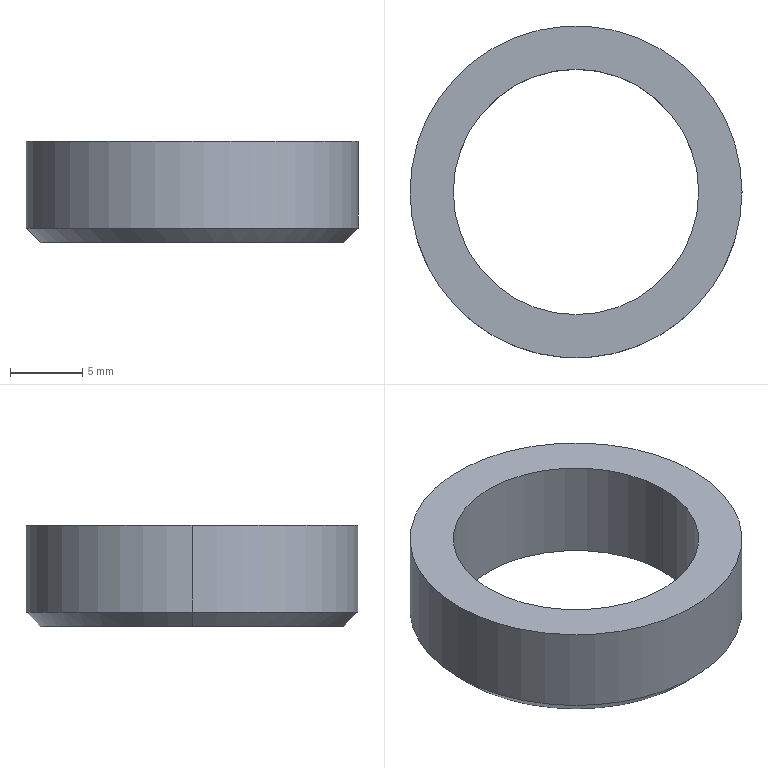Part | NX | features BREP 1 | 1 solid | 8 faces | box 23 x 23 x 7 mm | volume 1284 mm3 | cylinder 4 | cone 2 | plane 2 | commonest cylinder face diameters 17 x2 23 x2
STEP:
#1=CARTESIAN_POINT('',(-11.5,0.,-6.));
#2=VERTEX_POINT('',#1);
#3=CARTESIAN_POINT('',(-11.5,0.,0.));
#4=VERTEX_POINT('',#3);
#5=CARTESIAN_POINT('',(-11.5,0.,0.));
#6=DIRECTION('',(0.,0.,-1.));
#7=VECTOR('',#6,1000.);
#8=LINE('',#5,#7);
#9=EDGE_CURVE('',#2,#4,#8,.F.);
#10=ORIENTED_EDGE('',*,*,#9,.T.);
#11=CARTESIAN_POINT('',(11.5,0.,0.));
#12=VERTEX_POINT('',#11);
#13=CARTESIAN_POINT('',(0.,0.,0.));
#14=DIRECTION('',(0.,0.,1.));
#15=DIRECTION('',(1.,0.,0.));
#16=AXIS2_PLACEMENT_3D('',#13,#14,#15);
#17=CIRCLE('',#16,11.5);
#18=EDGE_CURVE('',#12,#4,#17,.T.);
#19=ORIENTED_EDGE('',*,*,#18,.F.);
#20=CARTESIAN_POINT('',(11.5,0.,-6.));
#21=VERTEX_POINT('',#20);
#22=CARTESIAN_POINT('',(11.5,0.,0.));
#23=DIRECTION('',(0.,0.,-1.));
#24=VECTOR('',#23,1000.);
#25=LINE('',#22,#24);
#26=EDGE_CURVE('',#21,#12,#25,.F.);
#27=ORIENTED_EDGE('',*,*,#26,.F.);
#28=CARTESIAN_POINT('',(0.,0.,-6.));
#29=DIRECTION('',(0.,0.,-1.));
#30=DIRECTION('',(-1.,0.,0.));
#31=AXIS2_PLACEMENT_3D('',#28,#29,#30);
#32=CIRCLE('',#31,11.5);
#33=EDGE_CURVE('',#2,#21,#32,.T.);
#34=ORIENTED_EDGE('',*,*,#33,.F.);
#35=EDGE_LOOP('',(#10,#19,#27,#34));
#36=FACE_BOUND('',#35,.T.);
#37=CARTESIAN_POINT('',(0.,0.,-7.));
#38=DIRECTION('',(0.,0.,1.));
#39=DIRECTION('',(-1.,0.,0.));
#40=AXIS2_PLACEMENT_3D('',#37,#38,#39);
#41=CYLINDRICAL_SURFACE('',#40,11.5);
#42=ADVANCED_FACE('',(#36),#41,.T.);
#43=CARTESIAN_POINT('',(-10.5,0.,-7.));
#44=VERTEX_POINT('',#43);
#45=CARTESIAN_POINT('',(-11.5,0.,-6.));
#46=DIRECTION('',(0.7071,0.,-0.7071));
#47=VECTOR('',#46,1000.);
#48=LINE('',#45,#47);
#49=EDGE_CURVE('',#44,#2,#48,.F.);
#50=ORIENTED_EDGE('',*,*,#49,.T.);
#51=ORIENTED_EDGE('',*,*,#33,.T.);
#52=CARTESIAN_POINT('',(10.5,0.,-7.));
#53=VERTEX_POINT('',#52);
#54=CARTESIAN_POINT('',(11.5,0.,-6.));
#55=DIRECTION('',(-0.7071,0.,-0.7071));
#56=VECTOR('',#55,1000.);
#57=LINE('',#54,#56);
#58=EDGE_CURVE('',#53,#21,#57,.F.);
#59=ORIENTED_EDGE('',*,*,#58,.F.);
#60=CARTESIAN_POINT('',(0.,0.,-7.));
#61=DIRECTION('',(0.,0.,-1.));
#62=DIRECTION('',(-1.,0.,0.));
#63=AXIS2_PLACEMENT_3D('',#60,#61,#62);
#64=CIRCLE('',#63,10.5);
#65=EDGE_CURVE('',#44,#53,#64,.T.);
#66=ORIENTED_EDGE('',*,*,#65,.F.);
#67=EDGE_LOOP('',(#50,#51,#59,#66));
#68=FACE_BOUND('',#67,.T.);
#69=CARTESIAN_POINT('',(0.,0.,-6.5));
#70=DIRECTION('',(0.,0.,1.));
#71=DIRECTION('',(-1.,0.,0.));
#72=AXIS2_PLACEMENT_3D('',#69,#70,#71);
#73=CONICAL_SURFACE('',#72,11.,0.7854);
#74=ADVANCED_FACE('',(#68),#73,.T.);
#75=ORIENTED_EDGE('',*,*,#65,.T.);
#76=CARTESIAN_POINT('',(0.,0.,-7.));
#77=DIRECTION('',(0.,0.,-1.));
#78=DIRECTION('',(1.,0.,0.));
#79=AXIS2_PLACEMENT_3D('',#76,#77,#78);
#80=CIRCLE('',#79,10.5);
#81=EDGE_CURVE('',#53,#44,#80,.T.);
#82=ORIENTED_EDGE('',*,*,#81,.T.);
#83=EDGE_LOOP('',(#75,#82));
#84=FACE_BOUND('',#83,.T.);
#85=CARTESIAN_POINT('',(8.5,0.,-7.));
#86=VERTEX_POINT('',#85);
#87=CARTESIAN_POINT('',(-8.5,0.,-7.));
#88=VERTEX_POINT('',#87);
#89=CARTESIAN_POINT('',(0.,0.,-7.));
#90=DIRECTION('',(0.,0.,1.));
#91=DIRECTION('',(1.,0.,0.));
#92=AXIS2_PLACEMENT_3D('',#89,#90,#91);
#93=CIRCLE('',#92,8.5);
#94=EDGE_CURVE('',#86,#88,#93,.T.);
#95=ORIENTED_EDGE('',*,*,#94,.T.);
#96=CARTESIAN_POINT('',(0.,0.,-7.));
#97=DIRECTION('',(0.,0.,1.));
#98=DIRECTION('',(-1.,0.,0.));
#99=AXIS2_PLACEMENT_3D('',#96,#97,#98);
#100=CIRCLE('',#99,8.5);
#101=EDGE_CURVE('',#88,#86,#100,.T.);
#102=ORIENTED_EDGE('',*,*,#101,.T.);
#103=EDGE_LOOP('',(#95,#102));
#104=FACE_BOUND('',#103,.T.);
#105=CARTESIAN_POINT('',(0.,0.,-7.));
#106=DIRECTION('',(0.,0.,-1.));
#107=DIRECTION('',(1.,0.,0.));
#108=AXIS2_PLACEMENT_3D('',#105,#106,#107);
#109=PLANE('',#108);
#110=ADVANCED_FACE('',(#84,#104),#109,.T.);
#111=ORIENTED_EDGE('',*,*,#81,.F.);
#112=ORIENTED_EDGE('',*,*,#58,.T.);
#113=CARTESIAN_POINT('',(0.,0.,-6.));
#114=DIRECTION('',(0.,0.,-1.));
#115=DIRECTION('',(1.,0.,0.));
#116=AXIS2_PLACEMENT_3D('',#113,#114,#115);
#117=CIRCLE('',#116,11.5);
#118=EDGE_CURVE('',#21,#2,#117,.T.);
#119=ORIENTED_EDGE('',*,*,#118,.T.);
#120=ORIENTED_EDGE('',*,*,#49,.F.);
#121=EDGE_LOOP('',(#111,#112,#119,#120));
#122=FACE_BOUND('',#121,.T.);
#123=CARTESIAN_POINT('',(0.,0.,-6.5));
#124=DIRECTION('',(0.,0.,1.));
#125=DIRECTION('',(-1.,0.,0.));
#126=AXIS2_PLACEMENT_3D('',#123,#124,#125);
#127=CONICAL_SURFACE('',#126,11.,0.7854);
#128=ADVANCED_FACE('',(#122),#127,.T.);
#129=ORIENTED_EDGE('',*,*,#118,.F.);
#130=ORIENTED_EDGE('',*,*,#26,.T.);
#131=CARTESIAN_POINT('',(0.,0.,0.));
#132=DIRECTION('',(0.,0.,1.));
#133=DIRECTION('',(-1.,0.,0.));
#134=AXIS2_PLACEMENT_3D('',#131,#132,#133);
#135=CIRCLE('',#134,11.5);
#136=EDGE_CURVE('',#4,#12,#135,.T.);
#137=ORIENTED_EDGE('',*,*,#136,.F.);
#138=ORIENTED_EDGE('',*,*,#9,.F.);
#139=EDGE_LOOP('',(#129,#130,#137,#138));
#140=FACE_BOUND('',#139,.T.);
#141=CARTESIAN_POINT('',(0.,0.,-7.));
#142=DIRECTION('',(0.,0.,1.));
#143=DIRECTION('',(-1.,0.,0.));
#144=AXIS2_PLACEMENT_3D('',#141,#142,#143);
#145=CYLINDRICAL_SURFACE('',#144,11.5);
#146=ADVANCED_FACE('',(#140),#145,.T.);
#147=ORIENTED_EDGE('',*,*,#18,.T.);
#148=ORIENTED_EDGE('',*,*,#136,.T.);
#149=EDGE_LOOP('',(#147,#148));
#150=FACE_BOUND('',#149,.T.);
#151=CARTESIAN_POINT('',(-8.5,0.,0.));
#152=VERTEX_POINT('',#151);
#153=CARTESIAN_POINT('',(8.5,0.,0.));
#154=VERTEX_POINT('',#153);
#155=CARTESIAN_POINT('',(0.,0.,0.));
#156=DIRECTION('',(0.,0.,-1.));
#157=DIRECTION('',(-1.,0.,0.));
#158=AXIS2_PLACEMENT_3D('',#155,#156,#157);
#159=CIRCLE('',#158,8.5);
#160=EDGE_CURVE('',#152,#154,#159,.T.);
#161=ORIENTED_EDGE('',*,*,#160,.T.);
#162=CARTESIAN_POINT('',(0.,0.,0.));
#163=DIRECTION('',(0.,0.,-1.));
#164=DIRECTION('',(1.,0.,0.));
#165=AXIS2_PLACEMENT_3D('',#162,#163,#164);
#166=CIRCLE('',#165,8.5);
#167=EDGE_CURVE('',#154,#152,#166,.T.);
#168=ORIENTED_EDGE('',*,*,#167,.T.);
#169=EDGE_LOOP('',(#161,#168));
#170=FACE_BOUND('',#169,.T.);
#171=CARTESIAN_POINT('',(0.,0.,0.));
#172=DIRECTION('',(0.,0.,-1.));
#173=DIRECTION('',(1.,0.,0.));
#174=AXIS2_PLACEMENT_3D('',#171,#172,#173);
#175=PLANE('',#174);
#176=ADVANCED_FACE('',(#150,#170),#175,.F.);
#177=CARTESIAN_POINT('',(-8.5,0.,0.));
#178=DIRECTION('',(0.,0.,-1.));
#179=VECTOR('',#178,1000.);
#180=LINE('',#177,#179);
#181=EDGE_CURVE('',#88,#152,#180,.F.);
#182=ORIENTED_EDGE('',*,*,#181,.T.);
#183=ORIENTED_EDGE('',*,*,#167,.F.);
#184=CARTESIAN_POINT('',(8.5,0.,0.));
#185=DIRECTION('',(0.,0.,-1.));
#186=VECTOR('',#185,1000.);
#187=LINE('',#184,#186);
#188=EDGE_CURVE('',#86,#154,#187,.F.);
#189=ORIENTED_EDGE('',*,*,#188,.F.);
#190=ORIENTED_EDGE('',*,*,#101,.F.);
#191=EDGE_LOOP('',(#182,#183,#189,#190));
#192=FACE_BOUND('',#191,.T.);
#193=CARTESIAN_POINT('',(0.,0.,-7.));
#194=DIRECTION('',(0.,0.,1.));
#195=DIRECTION('',(-1.,0.,0.));
#196=AXIS2_PLACEMENT_3D('',#193,#194,#195);
#197=CYLINDRICAL_SURFACE('',#196,8.5);
#198=ADVANCED_FACE('',(#192),#197,.F.);
#199=ORIENTED_EDGE('',*,*,#94,.F.);
#200=ORIENTED_EDGE('',*,*,#188,.T.);
#201=ORIENTED_EDGE('',*,*,#160,.F.);
#202=ORIENTED_EDGE('',*,*,#181,.F.);
#203=EDGE_LOOP('',(#199,#200,#201,#202));
#204=FACE_BOUND('',#203,.T.);
#205=CARTESIAN_POINT('',(0.,0.,-7.));
#206=DIRECTION('',(0.,0.,1.));
#207=DIRECTION('',(-1.,0.,0.));
#208=AXIS2_PLACEMENT_3D('',#205,#206,#207);
#209=CYLINDRICAL_SURFACE('',#208,8.5);
#210=ADVANCED_FACE('',(#204),#209,.F.);
#211=CLOSED_SHELL('',(#42,#74,#110,#128,#146,#176,#198,#210));
#212=MANIFOLD_SOLID_BREP('',#211);
#213=(LENGTH_UNIT()NAMED_UNIT(*)SI_UNIT(.MILLI.,.METRE.));
#214=UNCERTAINTY_MEASURE_WITH_UNIT(LENGTH_MEASURE(0.00001),#213,'','');
#215=(NAMED_UNIT(*)PLANE_ANGLE_UNIT()SI_UNIT($,.RADIAN.));
#216=(NAMED_UNIT(*)SI_UNIT($,.STERADIAN.)SOLID_ANGLE_UNIT());
#217=(GEOMETRIC_REPRESENTATION_CONTEXT(3)GLOBAL_UNCERTAINTY_ASSIGNED_CONTEXT((#214))GLOBAL_UNIT_ASSIGNED_CONTEXT((#213,#215,#216))REPRESENTATION_CONTEXT('',''));
#218=ADVANCED_BREP_SHAPE_REPRESENTATION('',(#212),#217);